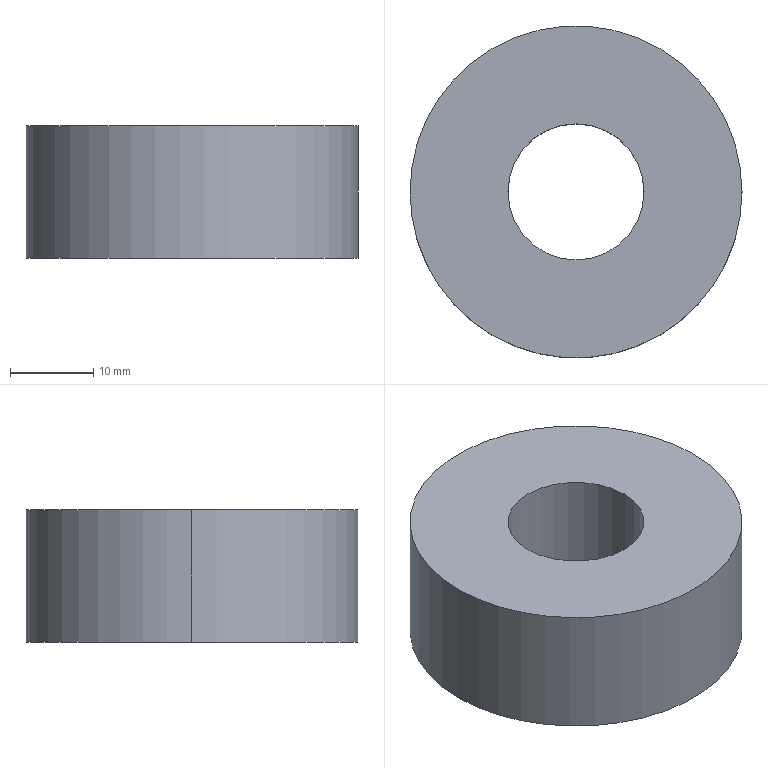Part | SolidWorks | features Extrusion 1 | 1 solid | 6 faces | box 40 x 40 x 16 mm | volume 16726 mm3 | cylinder 4 | plane 2 | commonest cylinder face diameters 16.4 x2 40 x2
STEP:
#1=CARTESIAN_POINT('',(-8.2,0.,-8.));
#2=VERTEX_POINT('',#1);
#3=CARTESIAN_POINT('',(8.2,0.,-8.));
#4=VERTEX_POINT('',#3);
#5=CARTESIAN_POINT('',(0.,0.,-8.));
#6=DIRECTION('',(0.,0.,1.));
#7=DIRECTION('',(1.,0.,0.));
#8=AXIS2_PLACEMENT_3D('',#5,#6,#7);
#9=CIRCLE('',#8,8.2);
#10=EDGE_CURVE('',#2,#4,#9,.T.);
#11=ORIENTED_EDGE('',*,*,#10,.F.);
#12=CARTESIAN_POINT('',(-8.2,0.,8.));
#13=VERTEX_POINT('',#12);
#14=CARTESIAN_POINT('',(-8.2,0.,-8.));
#15=DIRECTION('',(0.,0.,1.));
#16=VECTOR('',#15,1000.);
#17=LINE('',#14,#16);
#18=EDGE_CURVE('',#2,#13,#17,.T.);
#19=ORIENTED_EDGE('',*,*,#18,.T.);
#20=CARTESIAN_POINT('',(8.2,0.,8.));
#21=VERTEX_POINT('',#20);
#22=CARTESIAN_POINT('',(0.,0.,8.));
#23=DIRECTION('',(0.,0.,1.));
#24=DIRECTION('',(1.,0.,0.));
#25=AXIS2_PLACEMENT_3D('',#22,#23,#24);
#26=CIRCLE('',#25,8.2);
#27=EDGE_CURVE('',#13,#21,#26,.T.);
#28=ORIENTED_EDGE('',*,*,#27,.T.);
#29=CARTESIAN_POINT('',(8.2,0.,-8.));
#30=DIRECTION('',(0.,0.,1.));
#31=VECTOR('',#30,1000.);
#32=LINE('',#29,#31);
#33=EDGE_CURVE('',#4,#21,#32,.T.);
#34=ORIENTED_EDGE('',*,*,#33,.F.);
#35=EDGE_LOOP('',(#11,#19,#28,#34));
#36=FACE_OUTER_BOUND('',#35,.T.);
#37=CARTESIAN_POINT('',(0.,0.,-8.));
#38=DIRECTION('',(0.,0.,1.));
#39=DIRECTION('',(1.,0.,0.));
#40=AXIS2_PLACEMENT_3D('',#37,#38,#39);
#41=CYLINDRICAL_SURFACE('',#40,8.2);
#42=ADVANCED_FACE('',(#36),#41,.F.);
#43=CARTESIAN_POINT('',(20.,0.,-8.));
#44=VERTEX_POINT('',#43);
#45=CARTESIAN_POINT('',(-20.,0.,-8.));
#46=VERTEX_POINT('',#45);
#47=CARTESIAN_POINT('',(0.,0.,-8.));
#48=DIRECTION('',(0.,0.,1.));
#49=DIRECTION('',(1.,0.,0.));
#50=AXIS2_PLACEMENT_3D('',#47,#48,#49);
#51=CIRCLE('',#50,20.);
#52=EDGE_CURVE('',#44,#46,#51,.T.);
#53=ORIENTED_EDGE('',*,*,#52,.T.);
#54=CARTESIAN_POINT('',(-20.,0.,8.));
#55=VERTEX_POINT('',#54);
#56=CARTESIAN_POINT('',(-20.,0.,-8.));
#57=DIRECTION('',(0.,0.,1.));
#58=VECTOR('',#57,1000.);
#59=LINE('',#56,#58);
#60=EDGE_CURVE('',#46,#55,#59,.T.);
#61=ORIENTED_EDGE('',*,*,#60,.T.);
#62=CARTESIAN_POINT('',(20.,0.,8.));
#63=VERTEX_POINT('',#62);
#64=CARTESIAN_POINT('',(0.,0.,8.));
#65=DIRECTION('',(0.,0.,1.));
#66=DIRECTION('',(1.,0.,0.));
#67=AXIS2_PLACEMENT_3D('',#64,#65,#66);
#68=CIRCLE('',#67,20.);
#69=EDGE_CURVE('',#63,#55,#68,.T.);
#70=ORIENTED_EDGE('',*,*,#69,.F.);
#71=CARTESIAN_POINT('',(20.,0.,-8.));
#72=DIRECTION('',(0.,0.,1.));
#73=VECTOR('',#72,1000.);
#74=LINE('',#71,#73);
#75=EDGE_CURVE('',#44,#63,#74,.T.);
#76=ORIENTED_EDGE('',*,*,#75,.F.);
#77=EDGE_LOOP('',(#53,#61,#70,#76));
#78=FACE_OUTER_BOUND('',#77,.T.);
#79=CARTESIAN_POINT('',(0.,0.,-8.));
#80=DIRECTION('',(0.,0.,1.));
#81=DIRECTION('',(1.,0.,0.));
#82=AXIS2_PLACEMENT_3D('',#79,#80,#81);
#83=CYLINDRICAL_SURFACE('',#82,20.);
#84=ADVANCED_FACE('',(#78),#83,.T.);
#85=ORIENTED_EDGE('',*,*,#60,.F.);
#86=CARTESIAN_POINT('',(0.,0.,-8.));
#87=DIRECTION('',(0.,0.,1.));
#88=DIRECTION('',(1.,0.,0.));
#89=AXIS2_PLACEMENT_3D('',#86,#87,#88);
#90=CIRCLE('',#89,20.);
#91=EDGE_CURVE('',#46,#44,#90,.T.);
#92=ORIENTED_EDGE('',*,*,#91,.T.);
#93=ORIENTED_EDGE('',*,*,#75,.T.);
#94=CARTESIAN_POINT('',(0.,0.,8.));
#95=DIRECTION('',(0.,0.,1.));
#96=DIRECTION('',(1.,0.,0.));
#97=AXIS2_PLACEMENT_3D('',#94,#95,#96);
#98=CIRCLE('',#97,20.);
#99=EDGE_CURVE('',#55,#63,#98,.T.);
#100=ORIENTED_EDGE('',*,*,#99,.F.);
#101=EDGE_LOOP('',(#85,#92,#93,#100));
#102=FACE_OUTER_BOUND('',#101,.T.);
#103=CARTESIAN_POINT('',(0.,0.,-8.));
#104=DIRECTION('',(0.,0.,1.));
#105=DIRECTION('',(1.,0.,0.));
#106=AXIS2_PLACEMENT_3D('',#103,#104,#105);
#107=CYLINDRICAL_SURFACE('',#106,20.);
#108=ADVANCED_FACE('',(#102),#107,.T.);
#109=CARTESIAN_POINT('',(0.,0.,-8.));
#110=DIRECTION('',(0.,0.,1.));
#111=DIRECTION('',(1.,0.,0.));
#112=AXIS2_PLACEMENT_3D('',#109,#110,#111);
#113=CIRCLE('',#112,8.2);
#114=EDGE_CURVE('',#4,#2,#113,.T.);
#115=ORIENTED_EDGE('',*,*,#114,.T.);
#116=ORIENTED_EDGE('',*,*,#10,.T.);
#117=EDGE_LOOP('',(#115,#116));
#118=FACE_BOUND('',#117,.T.);
#119=ORIENTED_EDGE('',*,*,#52,.F.);
#120=ORIENTED_EDGE('',*,*,#91,.F.);
#121=EDGE_LOOP('',(#119,#120));
#122=FACE_OUTER_BOUND('',#121,.T.);
#123=CARTESIAN_POINT('',(0.,0.,-8.));
#124=DIRECTION('',(0.,0.,1.));
#125=DIRECTION('',(1.,0.,0.));
#126=AXIS2_PLACEMENT_3D('',#123,#124,#125);
#127=PLANE('',#126);
#128=ADVANCED_FACE('',(#118,#122),#127,.F.);
#129=CARTESIAN_POINT('',(0.,0.,8.));
#130=DIRECTION('',(0.,0.,1.));
#131=DIRECTION('',(1.,0.,0.));
#132=AXIS2_PLACEMENT_3D('',#129,#130,#131);
#133=CIRCLE('',#132,8.2);
#134=EDGE_CURVE('',#21,#13,#133,.T.);
#135=ORIENTED_EDGE('',*,*,#134,.F.);
#136=ORIENTED_EDGE('',*,*,#27,.F.);
#137=EDGE_LOOP('',(#135,#136));
#138=FACE_BOUND('',#137,.T.);
#139=ORIENTED_EDGE('',*,*,#69,.T.);
#140=ORIENTED_EDGE('',*,*,#99,.T.);
#141=EDGE_LOOP('',(#139,#140));
#142=FACE_OUTER_BOUND('',#141,.T.);
#143=CARTESIAN_POINT('',(0.,0.,8.));
#144=DIRECTION('',(0.,0.,1.));
#145=DIRECTION('',(1.,0.,0.));
#146=AXIS2_PLACEMENT_3D('',#143,#144,#145);
#147=PLANE('',#146);
#148=ADVANCED_FACE('',(#138,#142),#147,.T.);
#149=ORIENTED_EDGE('',*,*,#18,.F.);
#150=ORIENTED_EDGE('',*,*,#114,.F.);
#151=ORIENTED_EDGE('',*,*,#33,.T.);
#152=ORIENTED_EDGE('',*,*,#134,.T.);
#153=EDGE_LOOP('',(#149,#150,#151,#152));
#154=FACE_OUTER_BOUND('',#153,.T.);
#155=CARTESIAN_POINT('',(0.,0.,-8.));
#156=DIRECTION('',(0.,0.,1.));
#157=DIRECTION('',(1.,0.,0.));
#158=AXIS2_PLACEMENT_3D('',#155,#156,#157);
#159=CYLINDRICAL_SURFACE('',#158,8.2);
#160=ADVANCED_FACE('',(#154),#159,.F.);
#161=CLOSED_SHELL('',(#42,#84,#108,#128,#148,#160));
#162=MANIFOLD_SOLID_BREP('',#161);
#163=CARTESIAN_POINT('',(0.,0.,0.));
#164=DIRECTION('',(0.,0.,1.));
#165=DIRECTION('',(1.,0.,0.));
#166=AXIS2_PLACEMENT_3D('',#163,#164,#165);
#167=(LENGTH_UNIT()NAMED_UNIT(*)SI_UNIT(.MILLI.,.METRE.));
#168=UNCERTAINTY_MEASURE_WITH_UNIT(LENGTH_MEASURE(0.00001),#167,'','');
#169=(NAMED_UNIT(*)PLANE_ANGLE_UNIT()SI_UNIT($,.RADIAN.));
#170=(NAMED_UNIT(*)SI_UNIT($,.STERADIAN.)SOLID_ANGLE_UNIT());
#171=(GEOMETRIC_REPRESENTATION_CONTEXT(3)GLOBAL_UNCERTAINTY_ASSIGNED_CONTEXT((#168))GLOBAL_UNIT_ASSIGNED_CONTEXT((#167,#169,#170))REPRESENTATION_CONTEXT('',''));
#172=ADVANCED_BREP_SHAPE_REPRESENTATION('',(#162,#166),#171);